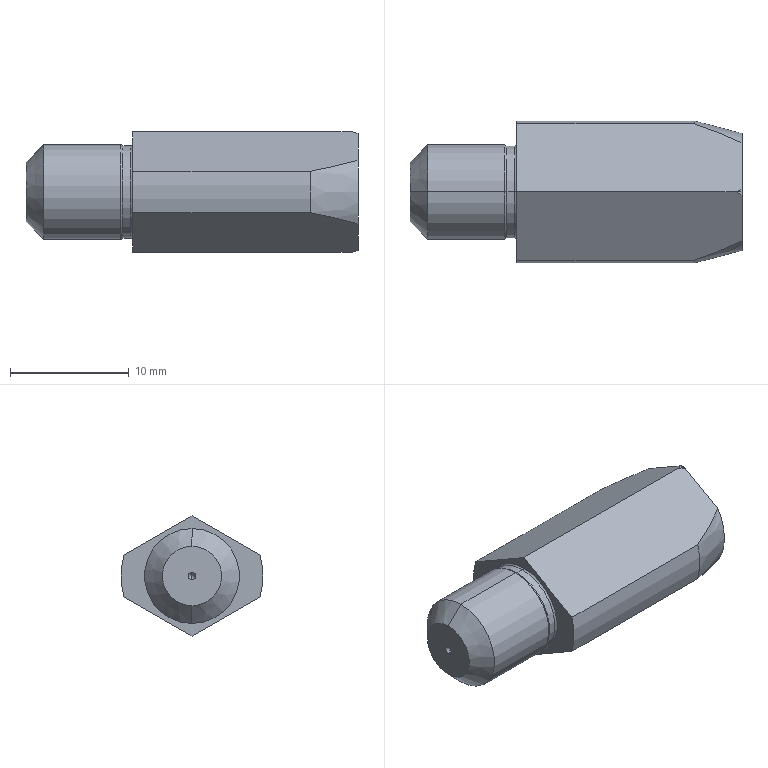Part | STEP file | FPBD8_P12_L9_B15_FPBD8-P12-L9-B15 | 1 solid | 28 faces | box 28 x 12 x 10.127 mm | volume 1917 mm3 | cone 11 | plane 7 | cylinder 6 | torus 4 | commonest cylinder face diameters 7.8 x2 8 x2 12 x2